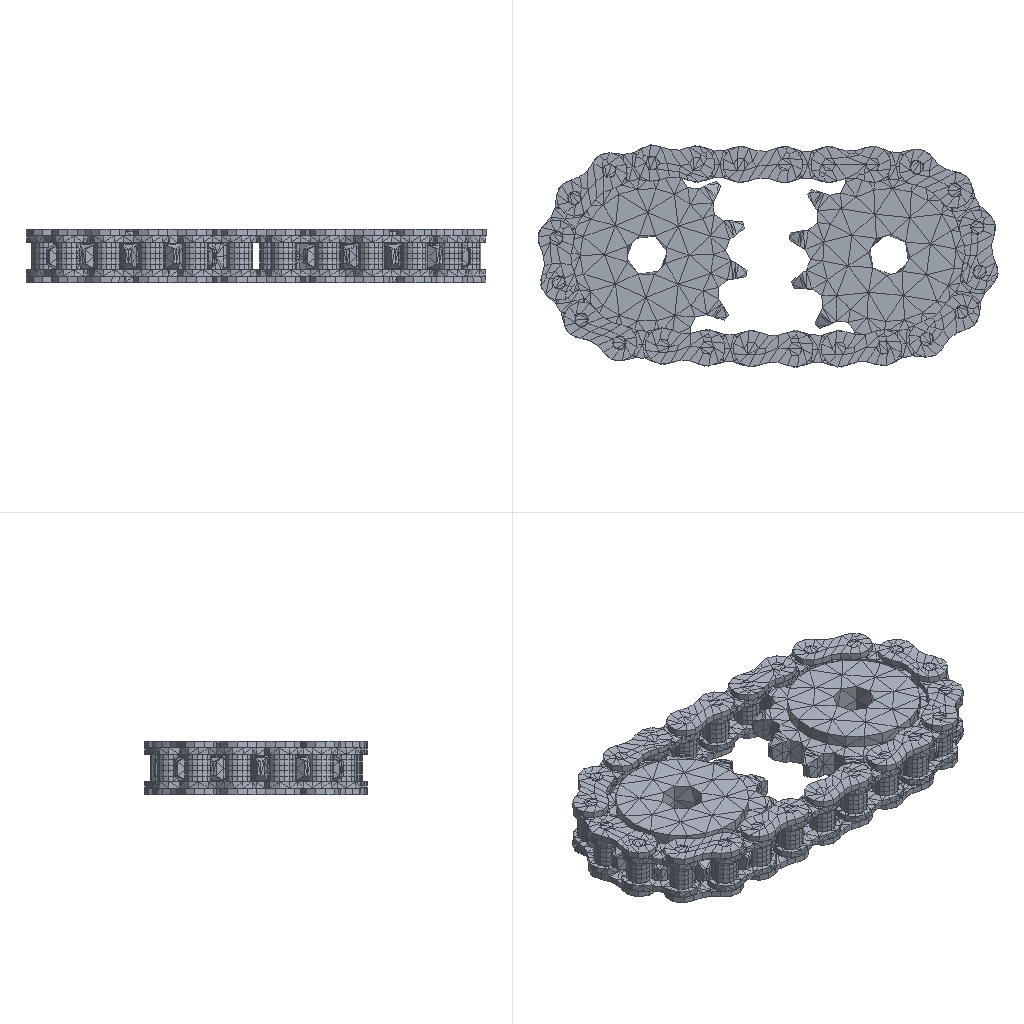Simulation study | ansys workbench
Set-up summary, first 216 of 799 lines:
category,name,step,type,value,unit,region
solver,ansys_mapdl
solver,version,,,22.1
solver,version,,,22.1
solver,version,,,22.1
solver,version,,,22.1
solver,version,,,22.1
units,MPA,,stated
analysis,deck1,,modal,modal
load_step,requested,,,1
analysis,nlgeom,,,False
mesh,nodes,,,40477
mesh,elements,,,27735
element_type,ANSYS 187 (type 1),,solid,1403
element_type,ANSYS 187 (type 2),,solid,1410
element_type,ANSYS 187 (type 3),,solid,507
element_type,ANSYS 186 (type 4),,solid,90
element_type,ANSYS 186 (type 5),,solid,90
element_type,ANSYS 186 (type 6),,solid,29
element_type,ANSYS 186 (type 7),,solid,24
element_type,ANSYS 187 (type 8),,solid,524
element_type,ANSYS 186 (type 9),,solid,90
element_type,ANSYS 186 (type 10),,solid,90
element_type,ANSYS 187 (type 11),,solid,506
element_type,ANSYS 186 (type 12),,solid,90
element_type,ANSYS 186 (type 13),,solid,90
element_type,ANSYS 186 (type 14),,solid,24
element_type,ANSYS 186 (type 15),,solid,31
element_type,ANSYS 186 (type 16),,solid,90
element_type,ANSYS 186 (type 17),,solid,90
element_type,ANSYS 187 (type 18),,solid,491
element_type,ANSYS 186 (type 19),,solid,23
element_type,ANSYS 186 (type 20),,solid,26
element_type,ANSYS 186 (type 21),,solid,31
element_type,ANSYS 186 (type 22),,solid,25
element_type,ANSYS 187 (type 23),,solid,506
element_type,ANSYS 186 (type 24),,solid,90
element_type,ANSYS 186 (type 25),,solid,90
element_type,ANSYS 186 (type 26),,solid,31
element_type,ANSYS 186 (type 27),,solid,25
element_type,ANSYS 186 (type 28),,solid,30
element_type,ANSYS 186 (type 29),,solid,23
element_type,ANSYS 187 (type 30),,solid,512
element_type,ANSYS 186 (type 31),,solid,90
element_type,ANSYS 186 (type 32),,solid,90
element_type,ANSYS 186 (type 33),,solid,25
element_type,ANSYS 186 (type 34),,solid,30
element_type,ANSYS 187 (type 35),,solid,516
element_type,ANSYS 186 (type 36),,solid,90
element_type,ANSYS 186 (type 37),,solid,90
element_type,ANSYS 186 (type 38),,solid,28
element_type,ANSYS 186 (type 39),,solid,24
element_type,ANSYS 187 (type 40),,solid,521
element_type,ANSYS 186 (type 41),,solid,90
element_type,ANSYS 186 (type 42),,solid,90
element_type,ANSYS 186 (type 43),,solid,24
element_type,ANSYS 186 (type 44),,solid,31
element_type,ANSYS 187 (type 45),,solid,497
element_type,ANSYS 186 (type 46),,solid,90
element_type,ANSYS 186 (type 47),,solid,90
element_type,ANSYS 186 (type 48),,solid,30
element_type,ANSYS 186 (type 49),,solid,24
element_type,ANSYS 187 (type 50),,solid,518
element_type,ANSYS 186 (type 51),,solid,90
element_type,ANSYS 186 (type 52),,solid,90
element_type,ANSYS 186 (type 53),,solid,25
element_type,ANSYS 186 (type 54),,solid,29
element_type,ANSYS 187 (type 55),,solid,516
element_type,ANSYS 186 (type 56),,solid,90
element_type,ANSYS 186 (type 57),,solid,90
element_type,ANSYS 187 (type 58),,solid,513
element_type,ANSYS 186 (type 59),,solid,90
element_type,ANSYS 186 (type 60),,solid,90
element_type,ANSYS 186 (type 61),,solid,30
element_type,ANSYS 186 (type 62),,solid,25
element_type,ANSYS 174 (type 63),,contact,42
element_type,ANSYS 170 (type 64),,target,42
element_type,ANSYS 174 (type 65),,contact,58
element_type,ANSYS 170 (type 66),,target,58
element_type,ANSYS 174 (type 67),,contact,58
element_type,ANSYS 170 (type 68),,target,58
element_type,ANSYS 174 (type 69),,contact,40
element_type,ANSYS 170 (type 70),,target,40
element_type,ANSYS 174 (type 71),,contact,58
element_type,ANSYS 170 (type 72),,target,58
element_type,ANSYS 174 (type 73),,contact,58
element_type,ANSYS 170 (type 74),,target,58
element_type,ANSYS 174 (type 75),,contact,43
element_type,ANSYS 170 (type 76),,target,43
element_type,ANSYS 174 (type 77),,contact,58
element_type,ANSYS 170 (type 78),,target,58
element_type,ANSYS 174 (type 79),,contact,58
element_type,ANSYS 170 (type 80),,target,58
element_type,ANSYS 174 (type 81),,contact,42
element_type,ANSYS 170 (type 82),,target,42
element_type,ANSYS 174 (type 83),,contact,58
element_type,ANSYS 170 (type 84),,target,58
element_type,ANSYS 174 (type 85),,contact,58
element_type,ANSYS 170 (type 86),,target,58
element_type,ANSYS 174 (type 87),,contact,8
element_type,ANSYS 170 (type 88),,target,8
element_type,ANSYS 174 (type 89),,contact,42
element_type,ANSYS 170 (type 90),,target,42
element_type,ANSYS 174 (type 91),,contact,58
element_type,ANSYS 170 (type 92),,target,58
element_type,ANSYS 174 (type 93),,contact,58
element_type,ANSYS 170 (type 94),,target,58
element_type,ANSYS 174 (type 95),,contact,40
element_type,ANSYS 170 (type 96),,target,40
element_type,ANSYS 174 (type 97),,contact,58
element_type,ANSYS 170 (type 98),,target,58
element_type,ANSYS 174 (type 99),,contact,58
element_type,ANSYS 170 (type 100),,target,58
element_type,ANSYS 174 (type 101),,contact,40
element_type,ANSYS 170 (type 102),,target,40
element_type,ANSYS 174 (type 103),,contact,58
element_type,ANSYS 170 (type 104),,target,58
element_type,ANSYS 174 (type 105),,contact,58
element_type,ANSYS 170 (type 106),,target,58
element_type,ANSYS 174 (type 107),,contact,58
element_type,ANSYS 170 (type 108),,target,58
element_type,ANSYS 174 (type 109),,contact,58
element_type,ANSYS 170 (type 110),,target,58
element_type,ANSYS 174 (type 111),,contact,40
element_type,ANSYS 170 (type 112),,target,40
element_type,ANSYS 174 (type 113),,contact,166
element_type,ANSYS 170 (type 114),,target,166
element_type,ANSYS 174 (type 115),,contact,150
element_type,ANSYS 170 (type 116),,target,150
element_type,ANSYS 174 (type 117),,contact,60
element_type,ANSYS 170 (type 118),,target,60
element_type,ANSYS 174 (type 119),,contact,57
element_type,ANSYS 170 (type 120),,target,57
element_type,ANSYS 174 (type 121),,contact,60
element_type,ANSYS 170 (type 122),,target,60
element_type,ANSYS 174 (type 123),,contact,64
element_type,ANSYS 170 (type 124),,target,64
element_type,ANSYS 174 (type 125),,contact,67
element_type,ANSYS 170 (type 126),,target,67
element_type,ANSYS 174 (type 127),,contact,65
element_type,ANSYS 170 (type 128),,target,65
element_type,ANSYS 174 (type 129),,contact,164
element_type,ANSYS 170 (type 130),,target,164
element_type,ANSYS 174 (type 131),,contact,152
element_type,ANSYS 170 (type 132),,target,152
element_type,ANSYS 174 (type 133),,contact,58
element_type,ANSYS 170 (type 134),,target,58
element_type,ANSYS 174 (type 135),,contact,59
element_type,ANSYS 170 (type 136),,target,59
element_type,ANSYS 174 (type 137),,contact,168
element_type,ANSYS 170 (type 138),,target,168
element_type,ANSYS 174 (type 139),,contact,152
element_type,ANSYS 170 (type 140),,target,152
element_type,ANSYS 174 (type 141),,contact,60
element_type,ANSYS 170 (type 142),,target,60
element_type,ANSYS 174 (type 143),,contact,68
element_type,ANSYS 170 (type 144),,target,68
element_type,ANSYS 174 (type 145),,contact,59
element_type,ANSYS 170 (type 146),,target,59
element_type,ANSYS 174 (type 147),,contact,60
element_type,ANSYS 170 (type 148),,target,60
element_type,ANSYS 174 (type 149),,contact,170
element_type,ANSYS 170 (type 150),,target,170
element_type,ANSYS 174 (type 151),,contact,152
element_type,ANSYS 170 (type 152),,target,152
element_type,ANSYS 174 (type 153),,contact,58
element_type,ANSYS 170 (type 154),,target,58
element_type,ANSYS 174 (type 155),,contact,59
element_type,ANSYS 170 (type 156),,target,59
element_type,ANSYS 174 (type 157),,contact,62
element_type,ANSYS 170 (type 158),,target,62
element_type,ANSYS 174 (type 159),,contact,63
element_type,ANSYS 170 (type 160),,target,63
element_type,ANSYS 174 (type 161),,contact,63
element_type,ANSYS 170 (type 162),,target,63
element_type,ANSYS 174 (type 163),,contact,56
element_type,ANSYS 170 (type 164),,target,56
element_type,ANSYS 174 (type 165),,contact,164
element_type,ANSYS 170 (type 166),,target,164
element_type,ANSYS 174 (type 167),,contact,150
element_type,ANSYS 170 (type 168),,target,150
element_type,ANSYS 174 (type 169),,contact,58
element_type,ANSYS 170 (type 170),,target,58
element_type,ANSYS 174 (type 171),,contact,56
element_type,ANSYS 170 (type 172),,target,56
element_type,ANSYS 174 (type 173),,contact,65
element_type,ANSYS 170 (type 174),,target,65
element_type,ANSYS 174 (type 175),,contact,61
element_type,ANSYS 170 (type 176),,target,61
element_type,ANSYS 174 (type 177),,contact,67
element_type,ANSYS 170 (type 178),,target,67
element_type,ANSYS 174 (type 179),,contact,63
element_type,ANSYS 170 (type 180),,target,63
element_type,ANSYS 174 (type 181),,contact,59
element_type,ANSYS 170 (type 182),,target,59
element_type,ANSYS 174 (type 183),,contact,60
element_type,ANSYS 170 (type 184),,target,60
element_type,ANSYS 174 (type 185),,contact,164
element_type,ANSYS 170 (type 186),,target,164
element_type,ANSYS 174 (type 187),,contact,152
element_type,ANSYS 170 (type 188),,target,152
element_type,ANSYS 174 (type 189),,contact,62
element_type,ANSYS 170 (type 190),,target,62
element_type,ANSYS 174 (type 191),,contact,69
element_type,ANSYS 170 (type 192),,target,69
element_type,ANSYS 174 (type 193),,contact,58
element_type,ANSYS 170 (type 194),,target,58
element_type,ANSYS 174 (type 195),,contact,56
element_type,ANSYS 170 (type 196),,target,56
element_type,ANSYS 174 (type 197),,contact,168
element_type,ANSYS 170 (type 198),,target,168
element_type,ANSYS 174 (type 199),,contact,152
element_type,ANSYS 170 (type 200),,target,152
element_type,ANSYS 174 (type 201),,contact,62
element_type,ANSYS 170 (type 202),,target,62
element_type,ANSYS 174 (type 203),,contact,62
Results summary:
result,analysis,,,modal
result,last_loadstep,,,1
result,primary field,,,displacement
result,reaction total,6,FX,228048.183,N
result,reaction total,6,FY,-1438789.858,N
result,reaction total,6,FZ,8343.782,N
result,analysis,,,modal
result,last_loadstep,,,1
result,primary field,,,displacement
result,analysis,,,modal
result,last_loadstep,,,1
result,primary field,,,displacement
result,reaction total,6,FX,228048.183,N
result,reaction total,6,FY,-1438789.858,N
result,reaction total,6,FZ,8343.782,N
result,analysis,,,spectrum
result,last_loadstep,,,5
result,primary field,,,displacement
result,reaction total,4,FX,748.064,N
result,reaction total,4,FY,977.567,N
result,reaction total,4,FZ,2265.835,N
result,analysis,,,static
result,last_loadstep,,,1
result,primary field,,,displacement
result,reaction total,1,FX,-0.0,N
result,reaction total,1,FY,0.0,N
result,reaction total,1,FZ,0.0,N
result,mass,,,0.008561,"NMM: mm, ton, N, s, mV, mA, degC"